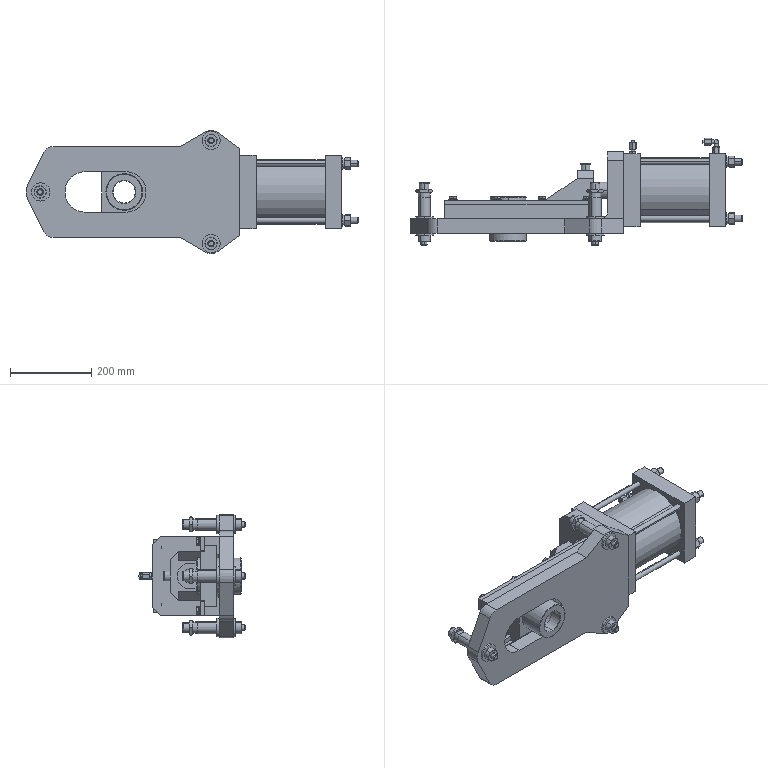Part | SolidWorks | features ReferencePattern 8, LocalLPattern 1, MirrorCompFeat 1 | 60 solids | 1331 faces | box 818.008 x 265.16 x 304.212 mm | volume 12071604 mm3 | plane 461 | cylinder 423 | cone 389 | torus 54 | sphere 3 | spline 1 | commonest cylinder face diameters 16 x38 10 x26 10.2 x24 16.182 x24 17 x24 45 x22